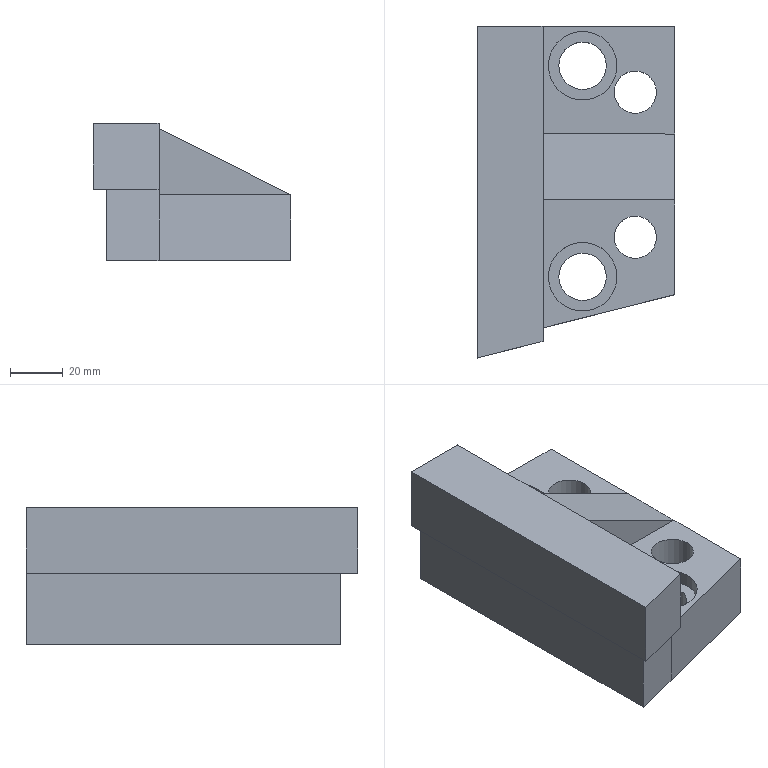Part | NX | features solid 2 | 1 solid | 24 faces | box 75 x 125.793 x 52 mm | volume 264906 mm3 | plane 15 | cylinder 6 | spline 3 | commonest cylinder face diameters 16 x2 18 x2 26 x2
STEP:
#1=CARTESIAN_POINT('',(-241.,585.,-55.));
#2=VERTEX_POINT('',#1);
#3=CARTESIAN_POINT('',(-250.,585.,-55.));
#4=DIRECTION('',(0.,0.,1.));
#5=DIRECTION('',(1.,0.,0.));
#6=AXIS2_PLACEMENT_3D('',#3,#4,#5);
#7=CIRCLE('',#6,9.);
#8=EDGE_CURVE('',#2,#2,#7,.T.);
#9=ORIENTED_EDGE('',*,*,#8,.F.);
#10=EDGE_LOOP('',(#9));
#11=FACE_BOUND('',#10,.T.);
#12=CARTESIAN_POINT('',(-241.,585.,-35.));
#13=VERTEX_POINT('',#12);
#14=CARTESIAN_POINT('',(-250.,585.,-35.));
#15=DIRECTION('',(0.,0.,1.));
#16=DIRECTION('',(1.,0.,0.));
#17=AXIS2_PLACEMENT_3D('',#14,#15,#16);
#18=CIRCLE('',#17,9.);
#19=EDGE_CURVE('',#13,#13,#18,.F.);
#20=ORIENTED_EDGE('',*,*,#19,.F.);
#21=EDGE_LOOP('',(#20));
#22=FACE_BOUND('',#21,.T.);
#23=CARTESIAN_POINT('',(-250.,585.,-60.));
#24=DIRECTION('',(0.,0.,1.));
#25=DIRECTION('',(1.,0.,0.));
#26=AXIS2_PLACEMENT_3D('',#23,#24,#25);
#27=CYLINDRICAL_SURFACE('',#26,9.);
#28=ADVANCED_FACE('',(#11,#22),#27,.F.);
#29=CARTESIAN_POINT('',(-241.,505.,-55.));
#30=VERTEX_POINT('',#29);
#31=CARTESIAN_POINT('',(-250.,505.,-55.));
#32=DIRECTION('',(0.,0.,1.));
#33=DIRECTION('',(1.,0.,0.));
#34=AXIS2_PLACEMENT_3D('',#31,#32,#33);
#35=CIRCLE('',#34,9.);
#36=EDGE_CURVE('',#30,#30,#35,.T.);
#37=ORIENTED_EDGE('',*,*,#36,.F.);
#38=EDGE_LOOP('',(#37));
#39=FACE_BOUND('',#38,.T.);
#40=CARTESIAN_POINT('',(-241.,505.,-35.));
#41=VERTEX_POINT('',#40);
#42=CARTESIAN_POINT('',(-250.,505.,-35.));
#43=DIRECTION('',(0.,0.,1.));
#44=DIRECTION('',(1.,0.,0.));
#45=AXIS2_PLACEMENT_3D('',#42,#43,#44);
#46=CIRCLE('',#45,9.);
#47=EDGE_CURVE('',#41,#41,#46,.F.);
#48=ORIENTED_EDGE('',*,*,#47,.F.);
#49=EDGE_LOOP('',(#48));
#50=FACE_BOUND('',#49,.T.);
#51=CARTESIAN_POINT('',(-250.,505.,-60.));
#52=DIRECTION('',(0.,0.,1.));
#53=DIRECTION('',(1.,0.,0.));
#54=AXIS2_PLACEMENT_3D('',#51,#52,#53);
#55=CYLINDRICAL_SURFACE('',#54,9.);
#56=ADVANCED_FACE('',(#39,#50),#55,.F.);
#57=CARTESIAN_POINT('',(-237.,505.,-30.));
#58=VERTEX_POINT('',#57);
#59=CARTESIAN_POINT('',(-250.,505.,-30.));
#60=DIRECTION('',(0.,0.,1.));
#61=DIRECTION('',(1.,0.,0.));
#62=AXIS2_PLACEMENT_3D('',#59,#60,#61);
#63=CIRCLE('',#62,13.);
#64=EDGE_CURVE('',#58,#58,#63,.T.);
#65=ORIENTED_EDGE('',*,*,#64,.F.);
#66=EDGE_LOOP('',(#65));
#67=FACE_BOUND('',#66,.T.);
#68=CARTESIAN_POINT('',(-222.,520.,-30.));
#69=VERTEX_POINT('',#68);
#70=CARTESIAN_POINT('',(-230.,520.,-30.));
#71=DIRECTION('',(0.,0.,1.));
#72=DIRECTION('',(1.,0.,0.));
#73=AXIS2_PLACEMENT_3D('',#70,#71,#72);
#74=CIRCLE('',#73,8.);
#75=EDGE_CURVE('',#69,#69,#74,.T.);
#76=ORIENTED_EDGE('',*,*,#75,.F.);
#77=EDGE_LOOP('',(#76));
#78=FACE_BOUND('',#77,.T.);
#79=CARTESIAN_POINT('',(-215.,534.109,-30.));
#80=VERTEX_POINT('',#79);
#81=CARTESIAN_POINT('',(-265.,534.109,-30.));
#82=VERTEX_POINT('',#81);
#83=CARTESIAN_POINT('',(-215.,534.109,-30.));
#84=DIRECTION('',(-1.,0.,0.));
#85=VECTOR('',#84,1000.);
#86=LINE('',#83,#85);
#87=EDGE_CURVE('',#80,#82,#86,.T.);
#88=ORIENTED_EDGE('',*,*,#87,.T.);
#89=CARTESIAN_POINT('',(-265.,485.664,-30.));
#90=VERTEX_POINT('',#89);
#91=CARTESIAN_POINT('',(-265.,487.395,-30.));
#92=DIRECTION('',(0.,1.,0.));
#93=VECTOR('',#92,1000.);
#94=LINE('',#91,#93);
#95=EDGE_CURVE('',#90,#82,#94,.T.);
#96=ORIENTED_EDGE('',*,*,#95,.F.);
#97=CARTESIAN_POINT('',(-215.,498.218,-30.));
#98=VERTEX_POINT('',#97);
#99=CARTESIAN_POINT('',(-265.,485.664,-30.));
#100=CARTESIAN_POINT('',(-248.333,489.849,-30.));
#101=CARTESIAN_POINT('',(-231.667,494.034,-30.));
#102=CARTESIAN_POINT('',(-215.,498.218,-30.));
#103=B_SPLINE_CURVE_WITH_KNOTS('',3,(#99,#100,#101,#102),.UNSPECIFIED.,.F.,.F.,(4,4),(0.1453,0.1968),.UNSPECIFIED.);
#104=EDGE_CURVE('',#90,#98,#103,.T.);
#105=ORIENTED_EDGE('',*,*,#104,.T.);
#106=CARTESIAN_POINT('',(-215.,487.395,-30.));
#107=DIRECTION('',(0.,1.,0.));
#108=VECTOR('',#107,1000.);
#109=LINE('',#106,#108);
#110=EDGE_CURVE('',#98,#80,#109,.T.);
#111=ORIENTED_EDGE('',*,*,#110,.T.);
#112=EDGE_LOOP('',(#88,#96,#105,#111));
#113=FACE_BOUND('',#112,.T.);
#114=CARTESIAN_POINT('',(-237.5,487.395,-30.));
#115=DIRECTION('',(0.,0.,1.));
#116=DIRECTION('',(1.,0.,0.));
#117=AXIS2_PLACEMENT_3D('',#114,#115,#116);
#118=PLANE('',#117);
#119=ADVANCED_FACE('',(#67,#78,#113),#118,.T.);
#120=CARTESIAN_POINT('',(-222.,575.,-55.));
#121=VERTEX_POINT('',#120);
#122=CARTESIAN_POINT('',(-230.,575.,-55.));
#123=DIRECTION('',(0.,0.,1.));
#124=DIRECTION('',(1.,0.,0.));
#125=AXIS2_PLACEMENT_3D('',#122,#123,#124);
#126=CIRCLE('',#125,8.);
#127=EDGE_CURVE('',#121,#121,#126,.T.);
#128=ORIENTED_EDGE('',*,*,#127,.T.);
#129=EDGE_LOOP('',(#128));
#130=FACE_BOUND('',#129,.T.);
#131=CARTESIAN_POINT('',(-222.,520.,-55.));
#132=VERTEX_POINT('',#131);
#133=CARTESIAN_POINT('',(-230.,520.,-55.));
#134=DIRECTION('',(0.,0.,1.));
#135=DIRECTION('',(1.,0.,0.));
#136=AXIS2_PLACEMENT_3D('',#133,#134,#135);
#137=CIRCLE('',#136,8.);
#138=EDGE_CURVE('',#132,#132,#137,.T.);
#139=ORIENTED_EDGE('',*,*,#138,.T.);
#140=EDGE_LOOP('',(#139));
#141=FACE_BOUND('',#140,.T.);
#142=ORIENTED_EDGE('',*,*,#8,.T.);
#143=EDGE_LOOP('',(#142));
#144=FACE_BOUND('',#143,.T.);
#145=ORIENTED_EDGE('',*,*,#36,.T.);
#146=EDGE_LOOP('',(#145));
#147=FACE_BOUND('',#146,.T.);
#148=CARTESIAN_POINT('',(-285.,480.629,-55.));
#149=VERTEX_POINT('',#148);
#150=CARTESIAN_POINT('',(-285.,600.,-55.));
#151=VERTEX_POINT('',#150);
#152=CARTESIAN_POINT('',(-285.,474.207,-55.));
#153=DIRECTION('',(0.,1.,0.));
#154=VECTOR('',#153,1000.);
#155=LINE('',#152,#154);
#156=EDGE_CURVE('',#149,#151,#155,.T.);
#157=ORIENTED_EDGE('',*,*,#156,.T.);
#158=CARTESIAN_POINT('',(-215.,600.,-55.));
#159=VERTEX_POINT('',#158);
#160=CARTESIAN_POINT('',(-277.501,600.,-55.));
#161=DIRECTION('',(-1.,0.,0.));
#162=VECTOR('',#161,1000.);
#163=LINE('',#160,#162);
#164=EDGE_CURVE('',#159,#151,#163,.T.);
#165=ORIENTED_EDGE('',*,*,#164,.F.);
#166=CARTESIAN_POINT('',(-215.,498.218,-55.));
#167=VERTEX_POINT('',#166);
#168=CARTESIAN_POINT('',(-215.,477.364,-55.));
#169=DIRECTION('',(0.,1.,0.));
#170=VECTOR('',#169,1000.);
#171=LINE('',#168,#170);
#172=EDGE_CURVE('',#167,#159,#171,.T.);
#173=ORIENTED_EDGE('',*,*,#172,.F.);
#174=CARTESIAN_POINT('',(-265.,485.664,-55.));
#175=VERTEX_POINT('',#174);
#176=CARTESIAN_POINT('',(-265.,485.664,-55.));
#177=CARTESIAN_POINT('',(-248.333,489.849,-55.));
#178=CARTESIAN_POINT('',(-231.667,494.034,-55.));
#179=CARTESIAN_POINT('',(-215.,498.218,-55.));
#180=B_SPLINE_CURVE_WITH_KNOTS('',3,(#176,#177,#178,#179),.UNSPECIFIED.,.F.,.F.,(4,4),(0.,0.05155),.UNSPECIFIED.);
#181=EDGE_CURVE('',#175,#167,#180,.T.);
#182=ORIENTED_EDGE('',*,*,#181,.F.);
#183=CARTESIAN_POINT('',(-265.,485.664,-55.));
#184=CARTESIAN_POINT('',(-271.667,483.986,-55.));
#185=CARTESIAN_POINT('',(-278.333,482.307,-55.));
#186=CARTESIAN_POINT('',(-285.,480.629,-55.));
#187=B_SPLINE_CURVE_WITH_KNOTS('',3,(#183,#184,#185,#186),.UNSPECIFIED.,.F.,.F.,(4,4),(0.,1.),.UNSPECIFIED.);
#188=EDGE_CURVE('',#149,#175,#187,.F.);
#189=ORIENTED_EDGE('',*,*,#188,.F.);
#190=EDGE_LOOP('',(#157,#165,#173,#182,#189));
#191=FACE_BOUND('',#190,.T.);
#192=CARTESIAN_POINT('',(-277.501,477.364,-55.));
#193=DIRECTION('',(0.,0.,1.));
#194=DIRECTION('',(1.,0.,0.));
#195=AXIS2_PLACEMENT_3D('',#192,#193,#194);
#196=PLANE('',#195);
#197=ADVANCED_FACE('',(#130,#141,#144,#147,#191),#196,.F.);
#198=CARTESIAN_POINT('',(-285.,480.629,-28.));
#199=VERTEX_POINT('',#198);
#200=CARTESIAN_POINT('',(-285.,480.629,-40.5));
#201=DIRECTION('',(0.,0.,-1.));
#202=VECTOR('',#201,1000.);
#203=LINE('',#200,#202);
#204=EDGE_CURVE('',#149,#199,#203,.F.);
#205=ORIENTED_EDGE('',*,*,#204,.F.);
#206=ORIENTED_EDGE('',*,*,#188,.T.);
#207=CARTESIAN_POINT('',(-265.,485.664,-40.5));
#208=DIRECTION('',(0.,0.,-1.));
#209=VECTOR('',#208,1000.);
#210=LINE('',#207,#209);
#211=EDGE_CURVE('',#175,#90,#210,.F.);
#212=ORIENTED_EDGE('',*,*,#211,.T.);
#213=CARTESIAN_POINT('',(-265.,485.664,-28.));
#214=VERTEX_POINT('',#213);
#215=CARTESIAN_POINT('',(-265.,485.664,-28.));
#216=DIRECTION('',(0.,0.,-1.));
#217=VECTOR('',#216,1000.);
#218=LINE('',#215,#217);
#219=EDGE_CURVE('',#214,#90,#218,.T.);
#220=ORIENTED_EDGE('',*,*,#219,.F.);
#221=CARTESIAN_POINT('',(-285.,480.629,-28.));
#222=CARTESIAN_POINT('',(-278.334,482.313,-28.));
#223=CARTESIAN_POINT('',(-271.665,483.99,-28.));
#224=CARTESIAN_POINT('',(-265.,485.664,-28.));
#225=B_SPLINE_CURVE_WITH_KNOTS('',3,(#221,#222,#223,#224),.UNSPECIFIED.,.F.,.F.,(4,4),(0.249,1.049),.UNSPECIFIED.);
#226=EDGE_CURVE('',#199,#214,#225,.T.);
#227=ORIENTED_EDGE('',*,*,#226,.F.);
#228=EDGE_LOOP('',(#205,#206,#212,#220,#227));
#229=FACE_BOUND('',#228,.T.);
#230=CARTESIAN_POINT('',(-285.,480.629,-28.));
#231=CARTESIAN_POINT('',(-285.,480.629,-55.));
#232=CARTESIAN_POINT('',(-278.334,482.313,-28.));
#233=CARTESIAN_POINT('',(-278.334,482.313,-55.));
#234=CARTESIAN_POINT('',(-271.665,483.99,-28.));
#235=CARTESIAN_POINT('',(-271.665,483.99,-55.));
#236=CARTESIAN_POINT('',(-265.,485.664,-28.));
#237=CARTESIAN_POINT('',(-265.,485.664,-55.));
#238=B_SPLINE_SURFACE_WITH_KNOTS('',3,1,((#230,#231),(#232,#233),(#234,#235),(#236,#237)),.SURF_OF_LINEAR_EXTRUSION.,.F.,.F.,.F.,(4,4),(2,2),(0.249,1.049),(0.,1.),.PIECEWISE_BEZIER_KNOTS.);
#239=ADVANCED_FACE('',(#229),#238,.F.);
#240=CARTESIAN_POINT('',(-290.,600.,-28.));
#241=VERTEX_POINT('',#240);
#242=CARTESIAN_POINT('',(-290.,600.,-3.));
#243=VERTEX_POINT('',#242);
#244=CARTESIAN_POINT('',(-290.,600.,-53.));
#245=DIRECTION('',(0.,0.,1.));
#246=VECTOR('',#245,1000.);
#247=LINE('',#244,#246);
#248=EDGE_CURVE('',#241,#243,#247,.T.);
#249=ORIENTED_EDGE('',*,*,#248,.F.);
#250=CARTESIAN_POINT('',(-290.,474.207,-28.));
#251=VERTEX_POINT('',#250);
#252=CARTESIAN_POINT('',(-290.,474.207,-28.));
#253=DIRECTION('',(0.,-1.,0.));
#254=VECTOR('',#253,1000.);
#255=LINE('',#252,#254);
#256=EDGE_CURVE('',#251,#241,#255,.F.);
#257=ORIENTED_EDGE('',*,*,#256,.F.);
#258=CARTESIAN_POINT('',(-290.,474.207,-3.));
#259=VERTEX_POINT('',#258);
#260=CARTESIAN_POINT('',(-290.,474.207,-53.));
#261=DIRECTION('',(0.,0.,1.));
#262=VECTOR('',#261,1000.);
#263=LINE('',#260,#262);
#264=EDGE_CURVE('',#251,#259,#263,.T.);
#265=ORIENTED_EDGE('',*,*,#264,.T.);
#266=CARTESIAN_POINT('',(-290.,474.207,-3.));
#267=DIRECTION('',(0.,1.,0.));
#268=VECTOR('',#267,1000.);
#269=LINE('',#266,#268);
#270=EDGE_CURVE('',#259,#243,#269,.T.);
#271=ORIENTED_EDGE('',*,*,#270,.T.);
#272=EDGE_LOOP('',(#249,#257,#265,#271));
#273=FACE_BOUND('',#272,.T.);
#274=CARTESIAN_POINT('',(-290.,474.207,-53.));
#275=DIRECTION('',(1.,0.,0.));
#276=DIRECTION('',(0.,0.,-1.));
#277=AXIS2_PLACEMENT_3D('',#274,#275,#276);
#278=PLANE('',#277);
#279=ADVANCED_FACE('',(#273),#278,.F.);
#280=CARTESIAN_POINT('',(-265.,534.109,-5.));
#281=VERTEX_POINT('',#280);
#282=CARTESIAN_POINT('',(-265.,534.109,-30.));
#283=DIRECTION('',(0.,0.,-1.));
#284=VECTOR('',#283,1000.);
#285=LINE('',#282,#284);
#286=EDGE_CURVE('',#281,#82,#285,.T.);
#287=ORIENTED_EDGE('',*,*,#286,.F.);
#288=CARTESIAN_POINT('',(-265.,559.109,-5.));
#289=VERTEX_POINT('',#288);
#290=CARTESIAN_POINT('',(-265.,534.109,-5.));
#291=DIRECTION('',(0.,1.,0.));
#292=VECTOR('',#291,1000.);
#293=LINE('',#290,#292);
#294=EDGE_CURVE('',#281,#289,#293,.T.);
#295=ORIENTED_EDGE('',*,*,#294,.T.);
#296=CARTESIAN_POINT('',(-265.,559.109,-30.));
#297=VERTEX_POINT('',#296);
#298=CARTESIAN_POINT('',(-265.,559.109,-30.));
#299=DIRECTION('',(0.,0.,1.));
#300=VECTOR('',#299,1000.);
#301=LINE('',#298,#300);
#302=EDGE_CURVE('',#289,#297,#301,.F.);
#303=ORIENTED_EDGE('',*,*,#302,.T.);
#304=CARTESIAN_POINT('',(-265.,600.,-30.));
#305=VERTEX_POINT('',#304);
#306=CARTESIAN_POINT('',(-265.,487.395,-30.));
#307=DIRECTION('',(0.,1.,0.));
#308=VECTOR('',#307,1000.);
#309=LINE('',#306,#308);
#310=EDGE_CURVE('',#297,#305,#309,.T.);
#311=ORIENTED_EDGE('',*,*,#310,.T.);
#312=CARTESIAN_POINT('',(-265.,600.,-3.));
#313=VERTEX_POINT('',#312);
#314=CARTESIAN_POINT('',(-265.,600.,-53.));
#315=DIRECTION('',(0.,0.,1.));
#316=VECTOR('',#315,1000.);
#317=LINE('',#314,#316);
#318=EDGE_CURVE('',#305,#313,#317,.T.);
#319=ORIENTED_EDGE('',*,*,#318,.T.);
#320=CARTESIAN_POINT('',(-265.,480.509,-3.));
#321=VERTEX_POINT('',#320);
#322=CARTESIAN_POINT('',(-265.,480.509,-3.));
#323=DIRECTION('',(0.,1.,0.));
#324=VECTOR('',#323,1000.);
#325=LINE('',#322,#324);
#326=EDGE_CURVE('',#321,#313,#325,.T.);
#327=ORIENTED_EDGE('',*,*,#326,.F.);
#328=CARTESIAN_POINT('',(-265.,480.509,-28.));
#329=VERTEX_POINT('',#328);
#330=CARTESIAN_POINT('',(-265.,480.509,-53.));
#331=DIRECTION('',(0.,0.,1.));
#332=VECTOR('',#331,1000.);
#333=LINE('',#330,#332);
#334=EDGE_CURVE('',#329,#321,#333,.T.);
#335=ORIENTED_EDGE('',*,*,#334,.F.);
#336=CARTESIAN_POINT('',(-265.,480.509,-28.));
#337=DIRECTION('',(0.,-1.,0.));
#338=VECTOR('',#337,1000.);
#339=LINE('',#336,#338);
#340=EDGE_CURVE('',#329,#214,#339,.F.);
#341=ORIENTED_EDGE('',*,*,#340,.T.);
#342=ORIENTED_EDGE('',*,*,#219,.T.);
#343=ORIENTED_EDGE('',*,*,#95,.T.);
#344=EDGE_LOOP('',(#287,#295,#303,#311,#319,#327,#335,#341,#342,#343));
#345=FACE_BOUND('',#344,.T.);
#346=CARTESIAN_POINT('',(-265.,480.509,-53.));
#347=DIRECTION('',(1.,0.,0.));
#348=DIRECTION('',(0.,0.,-1.));
#349=AXIS2_PLACEMENT_3D('',#346,#347,#348);
#350=PLANE('',#349);
#351=ADVANCED_FACE('',(#345),#350,.T.);
#352=CARTESIAN_POINT('',(-285.,600.,-28.));
#353=VERTEX_POINT('',#352);
#354=CARTESIAN_POINT('',(-265.,600.,-28.));
#355=DIRECTION('',(1.,0.,0.));
#356=VECTOR('',#355,1000.);
#357=LINE('',#354,#356);
#358=EDGE_CURVE('',#241,#353,#357,.T.);
#359=ORIENTED_EDGE('',*,*,#358,.F.);
#360=ORIENTED_EDGE('',*,*,#248,.T.);
#361=CARTESIAN_POINT('',(-265.,600.,-3.));
#362=DIRECTION('',(-1.,0.,0.));
#363=VECTOR('',#362,1000.);
#364=LINE('',#361,#363);
#365=EDGE_CURVE('',#313,#243,#364,.T.);
#366=ORIENTED_EDGE('',*,*,#365,.F.);
#367=ORIENTED_EDGE('',*,*,#318,.F.);
#368=CARTESIAN_POINT('',(-215.,600.,-30.));
#369=VERTEX_POINT('',#368);
#370=CARTESIAN_POINT('',(-237.5,600.,-30.));
#371=DIRECTION('',(-1.,0.,0.));
#372=VECTOR('',#371,1000.);
#373=LINE('',#370,#372);
#374=EDGE_CURVE('',#369,#305,#373,.T.);
#375=ORIENTED_EDGE('',*,*,#374,.F.);
#376=CARTESIAN_POINT('',(-215.,600.,-53.));
#377=DIRECTION('',(0.,0.,1.));
#378=VECTOR('',#377,1000.);
#379=LINE('',#376,#378);
#380=EDGE_CURVE('',#159,#369,#379,.T.);
#381=ORIENTED_EDGE('',*,*,#380,.F.);
#382=ORIENTED_EDGE('',*,*,#164,.T.);
#383=CARTESIAN_POINT('',(-285.,600.,-53.));
#384=DIRECTION('',(0.,0.,1.));
#385=VECTOR('',#384,1000.);
#386=LINE('',#383,#385);
#387=EDGE_CURVE('',#151,#353,#386,.T.);
#388=ORIENTED_EDGE('',*,*,#387,.T.);
#389=EDGE_LOOP('',(#359,#360,#366,#367,#375,#381,#382,#388));
#390=FACE_BOUND('',#389,.T.);
#391=CARTESIAN_POINT('',(-265.,600.,-53.));
#392=DIRECTION('',(0.,1.,0.));
#393=DIRECTION('',(0.,0.,1.));
#394=AXIS2_PLACEMENT_3D('',#391,#392,#393);
#395=PLANE('',#394);
#396=ADVANCED_FACE('',(#390),#395,.T.);
#397=CARTESIAN_POINT('',(-304.959,470.419,-28.));
#398=CARTESIAN_POINT('',(-302.847,470.954,-28.));
#399=CARTESIAN_POINT('',(-300.735,471.489,-28.));
#400=CARTESIAN_POINT('',(-298.623,472.024,-28.));
#401=CARTESIAN_POINT('',(-296.998,472.435,-28.));
#402=CARTESIAN_POINT('',(-295.374,472.846,-28.));
#403=CARTESIAN_POINT('',(-293.749,473.258,-28.));
#404=CARTESIAN_POINT('',(-292.499,473.574,-28.));
#405=CARTESIAN_POINT('',(-291.25,473.89,-28.));
#406=CARTESIAN_POINT('',(-290.,474.207,-28.));
#407=CARTESIAN_POINT('',(-281.669,476.316,-28.));
#408=CARTESIAN_POINT('',(-273.335,478.416,-28.));
#409=CARTESIAN_POINT('',(-265.,480.509,-28.));
#410=CARTESIAN_POINT('',(-263.75,480.823,-28.));
#411=CARTESIAN_POINT('',(-262.499,481.137,-28.));
#412=CARTESIAN_POINT('',(-261.249,481.451,-28.));
#413=CARTESIAN_POINT('',(-259.624,481.859,-28.));
#414=CARTESIAN_POINT('',(-257.998,482.267,-28.));
#415=CARTESIAN_POINT('',(-256.373,482.675,-28.));
#416=CARTESIAN_POINT('',(-254.26,483.206,-28.));
#417=CARTESIAN_POINT('',(-252.147,483.736,-28.));
#418=CARTESIAN_POINT('',(-250.034,484.267,-28.));
#419=B_SPLINE_CURVE_WITH_KNOTS('',3,(#397,#398,#399,#400,#401,#402,#403,#404,#405,#406,#407,#408,#409,#410,#411,#412,#413,#414,#415,#416,#417,#418),.UNSPECIFIED.,.F.,.F.,(4,3,3,3,3,3,3,4),(-0.5985,-0.345,-0.15,0.,1.,1.15,1.345,1.599),.PIECEWISE_BEZIER_KNOTS.);
#420=EDGE_CURVE('',#251,#329,#419,.T.);
#421=ORIENTED_EDGE('',*,*,#420,.T.);
#422=ORIENTED_EDGE('',*,*,#334,.T.);
#423=CARTESIAN_POINT('',(-290.,474.207,-3.));
#424=CARTESIAN_POINT('',(-281.669,476.316,-3.));
#425=CARTESIAN_POINT('',(-273.335,478.416,-3.));
#426=CARTESIAN_POINT('',(-265.,480.509,-3.));
#427=B_SPLINE_CURVE_WITH_KNOTS('',3,(#423,#424,#425,#426),.UNSPECIFIED.,.F.,.F.,(4,4),(0.,1.),.PIECEWISE_BEZIER_KNOTS.);
#428=EDGE_CURVE('',#259,#321,#427,.T.);
#429=ORIENTED_EDGE('',*,*,#428,.F.);
#430=ORIENTED_EDGE('',*,*,#264,.F.);
#431=EDGE_LOOP('',(#421,#422,#429,#430));
#432=FACE_BOUND('',#431,.T.);
#433=CARTESIAN_POINT('',(-290.,474.207,-28.));
#434=CARTESIAN_POINT('',(-290.,474.207,-3.));
#435=CARTESIAN_POINT('',(-281.669,476.316,-28.));
#436=CARTESIAN_POINT('',(-281.669,476.316,-3.));
#437=CARTESIAN_POINT('',(-273.335,478.416,-28.));
#438=CARTESIAN_POINT('',(-273.335,478.416,-3.));
#439=CARTESIAN_POINT('',(-265.,480.509,-28.));
#440=CARTESIAN_POINT('',(-265.,480.509,-3.));
#441=B_SPLINE_SURFACE_WITH_KNOTS('',3,1,((#433,#434),(#435,#436),(#437,#438),(#439,#440)),.SURF_OF_LINEAR_EXTRUSION.,.F.,.F.,.F.,(4,4),(2,2),(0.,1.),(0.,1.),.PIECEWISE_BEZIER_KNOTS.);
#442=ADVANCED_FACE('',(#432),#441,.T.);
#443=ORIENTED_EDGE('',*,*,#270,.F.);
#444=ORIENTED_EDGE('',*,*,#428,.T.);
#445=ORIENTED_EDGE('',*,*,#326,.T.);
#446=ORIENTED_EDGE('',*,*,#365,.T.);
#447=EDGE_LOOP('',(#443,#444,#445,#446));
#448=FACE_BOUND('',#447,.T.);
#449=CARTESIAN_POINT('',(-277.501,477.364,-3.));
#450=DIRECTION('',(0.,0.,1.));
#451=DIRECTION('',(1.,0.,0.));
#452=AXIS2_PLACEMENT_3D('',#449,#450,#451);
#453=PLANE('',#452);
#454=ADVANCED_FACE('',(#448),#453,.T.);
#455=CARTESIAN_POINT('',(-285.,474.207,-28.));
#456=DIRECTION('',(0.,1.,0.));
#457=VECTOR('',#456,1000.);
#458=LINE('',#455,#457);
#459=EDGE_CURVE('',#199,#353,#458,.T.);
#460=ORIENTED_EDGE('',*,*,#459,.F.);
#461=ORIENTED_EDGE('',*,*,#226,.T.);
#462=ORIENTED_EDGE('',*,*,#340,.F.);
#463=ORIENTED_EDGE('',*,*,#420,.F.);
#464=ORIENTED_EDGE('',*,*,#256,.T.);
#465=ORIENTED_EDGE('',*,*,#358,.T.);
#466=EDGE_LOOP('',(#460,#461,#462,#463,#464,#465));
#467=FACE_BOUND('',#466,.T.);
#468=CARTESIAN_POINT('',(-290.,474.207,-28.));
#469=DIRECTION('',(0.,0.,1.));
#470=DIRECTION('',(1.,0.,0.));
#471=AXIS2_PLACEMENT_3D('',#468,#469,#470);
#472=PLANE('',#471);
#473=ADVANCED_FACE('',(#467),#472,.F.);
#474=ORIENTED_EDGE('',*,*,#156,.F.);
#475=ORIENTED_EDGE('',*,*,#204,.T.);
#476=ORIENTED_EDGE('',*,*,#459,.T.);
#477=ORIENTED_EDGE('',*,*,#387,.F.);
#478=EDGE_LOOP('',(#474,#475,#476,#477));
#479=FACE_BOUND('',#478,.T.);
#480=CARTESIAN_POINT('',(-285.,474.207,-28.));
#481=DIRECTION('',(-1.,0.,0.));
#482=DIRECTION('',(0.,0.,1.));
#483=AXIS2_PLACEMENT_3D('',#480,#481,#482);
#484=PLANE('',#483);
#485=ADVANCED_FACE('',(#479),#484,.T.);
#486=ORIENTED_EDGE('',*,*,#110,.F.);
#487=CARTESIAN_POINT('',(-215.,498.218,-55.));
#488=DIRECTION('',(0.,0.,-1.));
#489=VECTOR('',#488,1000.);
#490=LINE('',#487,#489);
#491=EDGE_CURVE('',#167,#98,#490,.F.);
#492=ORIENTED_EDGE('',*,*,#491,.F.);
#493=ORIENTED_EDGE('',*,*,#172,.T.);
#494=ORIENTED_EDGE('',*,*,#380,.T.);
#495=CARTESIAN_POINT('',(-215.,559.109,-30.));
#496=VERTEX_POINT('',#495);
#497=CARTESIAN_POINT('',(-215.,487.395,-30.));
#498=DIRECTION('',(0.,1.,0.));
#499=VECTOR('',#498,1000.);
#500=LINE('',#497,#499);
#501=EDGE_CURVE('',#496,#369,#500,.T.);
#502=ORIENTED_EDGE('',*,*,#501,.F.);
#503=CARTESIAN_POINT('',(-215.,534.109,-30.));
#504=DIRECTION('',(0.,1.,0.));
#505=VECTOR('',#504,1000.);
#506=LINE('',#503,#505);
#507=EDGE_CURVE('',#80,#496,#506,.T.);
#508=ORIENTED_EDGE('',*,*,#507,.F.);
#509=EDGE_LOOP('',(#486,#492,#493,#494,#502,#508));
#510=FACE_BOUND('',#509,.T.);
#511=CARTESIAN_POINT('',(-215.,494.281,-53.));
#512=DIRECTION('',(1.,0.,0.));
#513=DIRECTION('',(0.,0.,-1.));
#514=AXIS2_PLACEMENT_3D('',#511,#512,#513);
#515=PLANE('',#514);
#516=ADVANCED_FACE('',(#510),#515,.T.);
#517=ORIENTED_EDGE('',*,*,#104,.F.);
#518=ORIENTED_EDGE('',*,*,#211,.F.);
#519=ORIENTED_EDGE('',*,*,#181,.T.);
#520=ORIENTED_EDGE('',*,*,#491,.T.);
#521=EDGE_LOOP('',(#517,#518,#519,#520));
#522=FACE_BOUND('',#521,.T.);
#523=CARTESIAN_POINT('',(-265.,485.664,-30.));
#524=CARTESIAN_POINT('',(-265.,485.664,-55.));
#525=CARTESIAN_POINT('',(-248.333,489.849,-30.));
#526=CARTESIAN_POINT('',(-248.333,489.849,-55.));
#527=CARTESIAN_POINT('',(-231.667,494.034,-30.));
#528=CARTESIAN_POINT('',(-231.667,494.034,-55.));
#529=CARTESIAN_POINT('',(-215.,498.218,-30.));
#530=CARTESIAN_POINT('',(-215.,498.218,-55.));
#531=B_SPLINE_SURFACE_WITH_KNOTS('',3,1,((#523,#524),(#525,#526),(#527,#528),(#529,#530)),.SURF_OF_LINEAR_EXTRUSION.,.F.,.F.,.F.,(4,4),(2,2),(0.,1.),(0.,1.),.PIECEWISE_BEZIER_KNOTS.);
#532=ADVANCED_FACE('',(#522),#531,.F.);
#533=CARTESIAN_POINT('',(-237.,585.,-30.));
#534=VERTEX_POINT('',#533);
#535=CARTESIAN_POINT('',(-250.,585.,-30.));
#536=DIRECTION('',(0.,0.,1.));
#537=DIRECTION('',(1.,0.,0.));
#538=AXIS2_PLACEMENT_3D('',#535,#536,#537);
#539=CIRCLE('',#538,13.);
#540=EDGE_CURVE('',#534,#534,#539,.T.);
#541=ORIENTED_EDGE('',*,*,#540,.F.);
#542=EDGE_LOOP('',(#541));
#543=FACE_BOUND('',#542,.T.);
#544=CARTESIAN_POINT('',(-222.,575.,-30.));
#545=VERTEX_POINT('',#544);
#546=CARTESIAN_POINT('',(-230.,575.,-30.));
#547=DIRECTION('',(0.,0.,1.));
#548=DIRECTION('',(1.,0.,0.));
#549=AXIS2_PLACEMENT_3D('',#546,#547,#548);
#550=CIRCLE('',#549,8.);
#551=EDGE_CURVE('',#545,#545,#550,.T.);
#552=ORIENTED_EDGE('',*,*,#551,.F.);
#553=EDGE_LOOP('',(#552));
#554=FACE_BOUND('',#553,.T.);
#555=CARTESIAN_POINT('',(-237.5,559.109,-30.));
#556=DIRECTION('',(1.,0.,0.));
#557=VECTOR('',#556,1000.);
#558=LINE('',#555,#557);
#559=EDGE_CURVE('',#496,#297,#558,.F.);
#560=ORIENTED_EDGE('',*,*,#559,.F.);
#561=ORIENTED_EDGE('',*,*,#501,.T.);
#562=ORIENTED_EDGE('',*,*,#374,.T.);
#563=ORIENTED_EDGE('',*,*,#310,.F.);
#564=EDGE_LOOP('',(#560,#561,#562,#563));
#565=FACE_BOUND('',#564,.T.);
#566=CARTESIAN_POINT('',(-237.5,487.395,-30.));
#567=DIRECTION('',(0.,0.,1.));
#568=DIRECTION('',(1.,0.,0.));
#569=AXIS2_PLACEMENT_3D('',#566,#567,#568);
#570=PLANE('',#569);
#571=ADVANCED_FACE('',(#543,#554,#565),#570,.T.);
#572=ORIENTED_EDGE('',*,*,#87,.F.);
#573=CARTESIAN_POINT('',(-215.,534.109,-30.));
#574=DIRECTION('',(0.8944,0.,-0.4472));
#575=VECTOR('',#574,1000.);
#576=LINE('',#573,#575);
#577=EDGE_CURVE('',#80,#281,#576,.F.);
#578=ORIENTED_EDGE('',*,*,#577,.T.);
#579=ORIENTED_EDGE('',*,*,#286,.T.);
#580=EDGE_LOOP('',(#572,#578,#579));
#581=FACE_BOUND('',#580,.T.);
#582=CARTESIAN_POINT('',(-215.,534.109,-30.));
#583=DIRECTION('',(0.,-1.,0.));
#584=DIRECTION('',(-1.,0.,0.));
#585=AXIS2_PLACEMENT_3D('',#582,#583,#584);
#586=PLANE('',#585);
#587=ADVANCED_FACE('',(#581),#586,.T.);
#588=ORIENTED_EDGE('',*,*,#302,.F.);
#589=CARTESIAN_POINT('',(-215.,559.109,-30.));
#590=DIRECTION('',(0.8944,0.,-0.4472));
#591=VECTOR('',#590,1000.);
#592=LINE('',#589,#591);
#593=EDGE_CURVE('',#289,#496,#592,.T.);
#594=ORIENTED_EDGE('',*,*,#593,.T.);
#595=ORIENTED_EDGE('',*,*,#559,.T.);
#596=EDGE_LOOP('',(#588,#594,#595));
#597=FACE_BOUND('',#596,.T.);
#598=CARTESIAN_POINT('',(-215.,559.109,-30.));
#599=DIRECTION('',(0.,-1.,0.));
#600=DIRECTION('',(-1.,0.,0.));
#601=AXIS2_PLACEMENT_3D('',#598,#599,#600);
#602=PLANE('',#601);
#603=ADVANCED_FACE('',(#597),#602,.F.);
#604=ORIENTED_EDGE('',*,*,#577,.F.);
#605=ORIENTED_EDGE('',*,*,#507,.T.);
#606=ORIENTED_EDGE('',*,*,#593,.F.);
#607=ORIENTED_EDGE('',*,*,#294,.F.);
#608=EDGE_LOOP('',(#604,#605,#606,#607));
#609=FACE_BOUND('',#608,.T.);
#610=CARTESIAN_POINT('',(-265.,534.109,-5.));
#611=DIRECTION('',(-0.4472,0.,-0.8944));
#612=DIRECTION('',(-0.8944,0.,0.4472));
#613=AXIS2_PLACEMENT_3D('',#610,#611,#612);
#614=PLANE('',#613);
#615=ADVANCED_FACE('',(#609),#614,.F.);
#616=ORIENTED_EDGE('',*,*,#75,.T.);
#617=EDGE_LOOP('',(#616));
#618=FACE_BOUND('',#617,.T.);
#619=ORIENTED_EDGE('',*,*,#138,.F.);
#620=EDGE_LOOP('',(#619));
#621=FACE_BOUND('',#620,.T.);
#622=CARTESIAN_POINT('',(-230.,520.,-60.));
#623=DIRECTION('',(0.,0.,1.));
#624=DIRECTION('',(1.,0.,0.));
#625=AXIS2_PLACEMENT_3D('',#622,#623,#624);
#626=CYLINDRICAL_SURFACE('',#625,8.);
#627=ADVANCED_FACE('',(#618,#621),#626,.F.);
#628=ORIENTED_EDGE('',*,*,#551,.T.);
#629=EDGE_LOOP('',(#628));
#630=FACE_BOUND('',#629,.T.);
#631=ORIENTED_EDGE('',*,*,#127,.F.);
#632=EDGE_LOOP('',(#631));
#633=FACE_BOUND('',#632,.T.);
#634=CARTESIAN_POINT('',(-230.,575.,-60.));
#635=DIRECTION('',(0.,0.,1.));
#636=DIRECTION('',(1.,0.,0.));
#637=AXIS2_PLACEMENT_3D('',#634,#635,#636);
#638=CYLINDRICAL_SURFACE('',#637,8.);
#639=ADVANCED_FACE('',(#630,#633),#638,.F.);
#640=CARTESIAN_POINT('',(-237.,505.,-35.));
#641=VERTEX_POINT('',#640);
#642=CARTESIAN_POINT('',(-250.,505.,-35.));
#643=DIRECTION('',(0.,0.,1.));
#644=DIRECTION('',(1.,0.,0.));
#645=AXIS2_PLACEMENT_3D('',#642,#643,#644);
#646=CIRCLE('',#645,13.);
#647=EDGE_CURVE('',#641,#641,#646,.T.);
#648=ORIENTED_EDGE('',*,*,#647,.T.);
#649=EDGE_LOOP('',(#648));
#650=FACE_BOUND('',#649,.T.);
#651=ORIENTED_EDGE('',*,*,#47,.T.);
#652=EDGE_LOOP('',(#651));
#653=FACE_BOUND('',#652,.T.);
#654=CARTESIAN_POINT('',(-250.,505.,-35.));
#655=DIRECTION('',(0.,0.,1.));
#656=DIRECTION('',(1.,0.,0.));
#657=AXIS2_PLACEMENT_3D('',#654,#655,#656);
#658=PLANE('',#657);
#659=ADVANCED_FACE('',(#650,#653),#658,.T.);
#660=ORIENTED_EDGE('',*,*,#647,.F.);
#661=EDGE_LOOP('',(#660));
#662=FACE_BOUND('',#661,.T.);
#663=ORIENTED_EDGE('',*,*,#64,.T.);
#664=EDGE_LOOP('',(#663));
#665=FACE_BOUND('',#664,.T.);
#666=CARTESIAN_POINT('',(-250.,505.,-35.));
#667=DIRECTION('',(0.,0.,1.));
#668=DIRECTION('',(1.,0.,0.));
#669=AXIS2_PLACEMENT_3D('',#666,#667,#668);
#670=CYLINDRICAL_SURFACE('',#669,13.);
#671=ADVANCED_FACE('',(#662,#665),#670,.F.);
#672=CARTESIAN_POINT('',(-237.,585.,-35.));
#673=VERTEX_POINT('',#672);
#674=CARTESIAN_POINT('',(-250.,585.,-35.));
#675=DIRECTION('',(0.,0.,1.));
#676=DIRECTION('',(1.,0.,0.));
#677=AXIS2_PLACEMENT_3D('',#674,#675,#676);
#678=CIRCLE('',#677,13.);
#679=EDGE_CURVE('',#673,#673,#678,.T.);
#680=ORIENTED_EDGE('',*,*,#679,.T.);
#681=EDGE_LOOP('',(#680));
#682=FACE_BOUND('',#681,.T.);
#683=ORIENTED_EDGE('',*,*,#19,.T.);
#684=EDGE_LOOP('',(#683));
#685=FACE_BOUND('',#684,.T.);
#686=CARTESIAN_POINT('',(-250.,585.,-35.));
#687=DIRECTION('',(0.,0.,1.));
#688=DIRECTION('',(1.,0.,0.));
#689=AXIS2_PLACEMENT_3D('',#686,#687,#688);
#690=PLANE('',#689);
#691=ADVANCED_FACE('',(#682,#685),#690,.T.);
#692=ORIENTED_EDGE('',*,*,#679,.F.);
#693=EDGE_LOOP('',(#692));
#694=FACE_BOUND('',#693,.T.);
#695=ORIENTED_EDGE('',*,*,#540,.T.);
#696=EDGE_LOOP('',(#695));
#697=FACE_BOUND('',#696,.T.);
#698=CARTESIAN_POINT('',(-250.,585.,-35.));
#699=DIRECTION('',(0.,0.,1.));
#700=DIRECTION('',(1.,0.,0.));
#701=AXIS2_PLACEMENT_3D('',#698,#699,#700);
#702=CYLINDRICAL_SURFACE('',#701,13.);
#703=ADVANCED_FACE('',(#694,#697),#702,.F.);
#704=CLOSED_SHELL('',(#28,#56,#119,#197,#239,#279,#351,#396,#442,#454,#473,#485,#516,#532,#571,#587,#603,#615,#627,#639,#659,#671,#691,#703));
#705=MANIFOLD_SOLID_BREP('',#704);
#706=(LENGTH_UNIT()NAMED_UNIT(*)SI_UNIT(.MILLI.,.METRE.));
#707=UNCERTAINTY_MEASURE_WITH_UNIT(LENGTH_MEASURE(0.0508),#706,'','');
#708=(NAMED_UNIT(*)PLANE_ANGLE_UNIT()SI_UNIT($,.RADIAN.));
#709=(NAMED_UNIT(*)SI_UNIT($,.STERADIAN.)SOLID_ANGLE_UNIT());
#710=(GEOMETRIC_REPRESENTATION_CONTEXT(3)GLOBAL_UNCERTAINTY_ASSIGNED_CONTEXT((#707))GLOBAL_UNIT_ASSIGNED_CONTEXT((#706,#708,#709))REPRESENTATION_CONTEXT('',''));
#711=ADVANCED_BREP_SHAPE_REPRESENTATION('',(#705),#710);